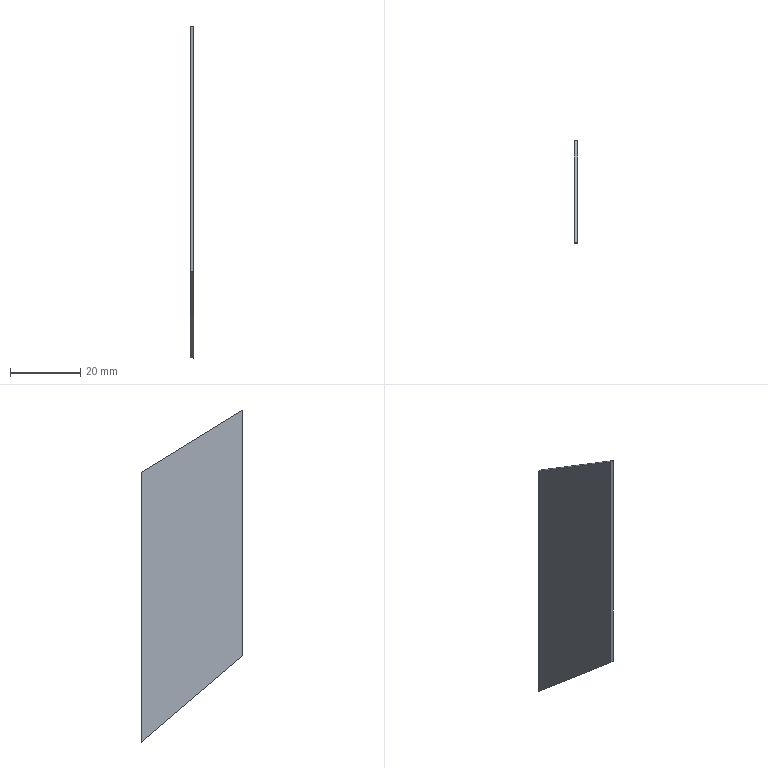Part | STEP file | 09-20 Outlet upper seal plate | 1 solid | 6 faces | box 1 x 29 x 94.448 mm | volume 2126 mm3 | plane 6
STEP:
#1=CARTESIAN_POINT('',(0.,0.,0.));
#2=DIRECTION('',(0.,0.,1.));
#3=DIRECTION('',(1.,0.,0.));
#4=AXIS2_PLACEMENT_3D('',#1,#2,#3);
#5=CARTESIAN_POINT('',(0.,0.,-69.892));
#6=VERTEX_POINT('',#5);
#7=CARTESIAN_POINT('',(1.,0.,-69.892));
#8=VERTEX_POINT('',#7);
#9=CARTESIAN_POINT('',(0.5,0.,-69.892));
#10=DIRECTION('',(1.,0.,0.));
#11=VECTOR('',#10,1.);
#12=LINE('',#9,#11);
#13=CARTESIAN_POINT('',(0.,0.,-69.892));
#14=DIRECTION('',(0.,1.,0.));
#15=DIRECTION('',(0.,0.,1.));
#16=AXIS2_PLACEMENT_3D('',#13,#14,#15);
#17=PLANE('',#16);
#18=CARTESIAN_POINT('',(0.,0.5));
#19=DIRECTION('',(0.,1.));
#20=VECTOR('',#19,1.);
#21=LINE('',#18,#20);
#22=(GEOMETRIC_REPRESENTATION_CONTEXT(2)PARAMETRIC_REPRESENTATION_CONTEXT()REPRESENTATION_CONTEXT('',''));
#23=DEFINITIONAL_REPRESENTATION('',(#21),#22);
#24=PCURVE('',#17,#23);
#25=CARTESIAN_POINT('',(0.,29.,-94.448));
#26=DIRECTION('',(0.,0.6462,0.7632));
#27=DIRECTION('',(0.,-0.7632,0.6462));
#28=AXIS2_PLACEMENT_3D('',#25,#26,#27);
#29=PLANE('',#28);
#30=CARTESIAN_POINT('',(38.,0.5));
#31=DIRECTION('',(0.,1.));
#32=VECTOR('',#31,1.);
#33=LINE('',#30,#32);
#34=(GEOMETRIC_REPRESENTATION_CONTEXT(2)PARAMETRIC_REPRESENTATION_CONTEXT()REPRESENTATION_CONTEXT('',''));
#35=DEFINITIONAL_REPRESENTATION('',(#33),#34);
#36=PCURVE('',#29,#35);
#37=SURFACE_CURVE('',#12,(#24,#36),.PCURVE_S1.);
#38=EDGE_CURVE('',#6,#8,#37,.T.);
#39=ORIENTED_EDGE('',*,*,#38,.T.);
#40=CARTESIAN_POINT('',(1.,0.,0.));
#41=VERTEX_POINT('',#40);
#42=CARTESIAN_POINT('',(1.,0.,-34.946));
#43=DIRECTION('',(0.,0.,-1.));
#44=VECTOR('',#43,1.);
#45=LINE('',#42,#44);
#46=CARTESIAN_POINT('',(34.946,1.));
#47=DIRECTION('',(-1.,0.));
#48=VECTOR('',#47,1.);
#49=LINE('',#46,#48);
#50=(GEOMETRIC_REPRESENTATION_CONTEXT(2)PARAMETRIC_REPRESENTATION_CONTEXT()REPRESENTATION_CONTEXT('',''));
#51=DEFINITIONAL_REPRESENTATION('',(#49),#50);
#52=PCURVE('',#17,#51);
#53=CARTESIAN_POINT('',(1.,0.,-95.015));
#54=DIRECTION('',(-1.,0.,0.));
#55=DIRECTION('',(0.,0.,1.));
#56=AXIS2_PLACEMENT_3D('',#53,#54,#55);
#57=PLANE('',#56);
#58=CARTESIAN_POINT('',(60.069,0.));
#59=DIRECTION('',(-1.,0.));
#60=VECTOR('',#59,1.);
#61=LINE('',#58,#60);
#62=(GEOMETRIC_REPRESENTATION_CONTEXT(2)PARAMETRIC_REPRESENTATION_CONTEXT()REPRESENTATION_CONTEXT('',''));
#63=DEFINITIONAL_REPRESENTATION('',(#61),#62);
#64=PCURVE('',#57,#63);
#65=SURFACE_CURVE('',#45,(#52,#64),.PCURVE_S1.);
#66=EDGE_CURVE('',#41,#8,#65,.T.);
#67=ORIENTED_EDGE('',*,*,#66,.F.);
#68=CARTESIAN_POINT('',(0.,0.,-0.000000012));
#69=VERTEX_POINT('',#68);
#70=CARTESIAN_POINT('',(0.5,0.,0.));
#71=DIRECTION('',(-1.,0.,0.));
#72=VECTOR('',#71,1.);
#73=LINE('',#70,#72);
#74=CARTESIAN_POINT('',(69.892,0.5));
#75=DIRECTION('',(0.,-1.));
#76=VECTOR('',#75,1.);
#77=LINE('',#74,#76);
#78=(GEOMETRIC_REPRESENTATION_CONTEXT(2)PARAMETRIC_REPRESENTATION_CONTEXT()REPRESENTATION_CONTEXT('',''));
#79=DEFINITIONAL_REPRESENTATION('',(#77),#78);
#80=PCURVE('',#17,#79);
#81=CARTESIAN_POINT('',(0.,0.,0.));
#82=DIRECTION('',(0.,-0.522,-0.8529));
#83=DIRECTION('',(0.,0.8529,-0.522));
#84=AXIS2_PLACEMENT_3D('',#81,#82,#83);
#85=PLANE('',#84);
#86=CARTESIAN_POINT('',(0.,0.5));
#87=DIRECTION('',(0.,-1.));
#88=VECTOR('',#87,1.);
#89=LINE('',#86,#88);
#90=(GEOMETRIC_REPRESENTATION_CONTEXT(2)PARAMETRIC_REPRESENTATION_CONTEXT()REPRESENTATION_CONTEXT('',''));
#91=DEFINITIONAL_REPRESENTATION('',(#89),#90);
#92=PCURVE('',#85,#91);
#93=SURFACE_CURVE('',#73,(#80,#92),.PCURVE_S1.);
#94=EDGE_CURVE('',#41,#69,#93,.T.);
#95=ORIENTED_EDGE('',*,*,#94,.T.);
#96=CARTESIAN_POINT('',(0.,0.,-34.946));
#97=DIRECTION('',(0.,0.,1.));
#98=VECTOR('',#97,1.);
#99=LINE('',#96,#98);
#100=CARTESIAN_POINT('',(34.946,0.));
#101=DIRECTION('',(1.,0.));
#102=VECTOR('',#101,1.);
#103=LINE('',#100,#102);
#104=(GEOMETRIC_REPRESENTATION_CONTEXT(2)PARAMETRIC_REPRESENTATION_CONTEXT()REPRESENTATION_CONTEXT('',''));
#105=DEFINITIONAL_REPRESENTATION('',(#103),#104);
#106=PCURVE('',#17,#105);
#107=CARTESIAN_POINT('',(0.,0.,-95.015));
#108=DIRECTION('',(-1.,0.,0.));
#109=DIRECTION('',(0.,0.,1.));
#110=AXIS2_PLACEMENT_3D('',#107,#108,#109);
#111=PLANE('',#110);
#112=CARTESIAN_POINT('',(60.069,0.));
#113=DIRECTION('',(1.,0.));
#114=VECTOR('',#113,1.);
#115=LINE('',#112,#114);
#116=(GEOMETRIC_REPRESENTATION_CONTEXT(2)PARAMETRIC_REPRESENTATION_CONTEXT()REPRESENTATION_CONTEXT('',''));
#117=DEFINITIONAL_REPRESENTATION('',(#115),#116);
#118=PCURVE('',#111,#117);
#119=SURFACE_CURVE('',#99,(#106,#118),.PCURVE_S1.);
#120=EDGE_CURVE('',#6,#69,#119,.T.);
#121=ORIENTED_EDGE('',*,*,#120,.F.);
#122=EDGE_LOOP('',(#39,#67,#95,#121));
#123=FACE_BOUND('',#122,.T.);
#124=ADVANCED_FACE('',(#123),#17,.F.);
#125=CARTESIAN_POINT('',(0.,29.,-17.748));
#126=VERTEX_POINT('',#125);
#127=CARTESIAN_POINT('',(0.,29.,-94.448));
#128=VERTEX_POINT('',#127);
#129=CARTESIAN_POINT('',(0.,29.,-47.224));
#130=DIRECTION('',(0.,0.,-1.));
#131=VECTOR('',#130,1.);
#132=LINE('',#129,#131);
#133=CARTESIAN_POINT('',(47.791,29.));
#134=DIRECTION('',(-1.,0.));
#135=VECTOR('',#134,1.);
#136=LINE('',#133,#135);
#137=(GEOMETRIC_REPRESENTATION_CONTEXT(2)PARAMETRIC_REPRESENTATION_CONTEXT()REPRESENTATION_CONTEXT('',''));
#138=DEFINITIONAL_REPRESENTATION('',(#136),#137);
#139=PCURVE('',#111,#138);
#140=CARTESIAN_POINT('',(0.,29.,-17.748));
#141=DIRECTION('',(0.,-1.,0.));
#142=DIRECTION('',(0.,0.,-1.));
#143=AXIS2_PLACEMENT_3D('',#140,#141,#142);
#144=PLANE('',#143);
#145=CARTESIAN_POINT('',(29.476,0.));
#146=DIRECTION('',(1.,0.));
#147=VECTOR('',#146,1.);
#148=LINE('',#145,#147);
#149=(GEOMETRIC_REPRESENTATION_CONTEXT(2)PARAMETRIC_REPRESENTATION_CONTEXT()REPRESENTATION_CONTEXT('',''));
#150=DEFINITIONAL_REPRESENTATION('',(#148),#149);
#151=PCURVE('',#144,#150);
#152=SURFACE_CURVE('',#132,(#139,#151),.PCURVE_S1.);
#153=EDGE_CURVE('',#126,#128,#152,.T.);
#154=ORIENTED_EDGE('',*,*,#153,.T.);
#155=CARTESIAN_POINT('',(0.,29.,-94.448));
#156=DIRECTION('',(0.,-0.7632,0.6462));
#157=VECTOR('',#156,1.);
#158=LINE('',#155,#157);
#159=CARTESIAN_POINT('',(0.5667,29.));
#160=DIRECTION('',(0.6462,-0.7632));
#161=VECTOR('',#160,1.);
#162=LINE('',#159,#161);
#163=(GEOMETRIC_REPRESENTATION_CONTEXT(2)PARAMETRIC_REPRESENTATION_CONTEXT()REPRESENTATION_CONTEXT('',''));
#164=DEFINITIONAL_REPRESENTATION('',(#162),#163);
#165=PCURVE('',#111,#164);
#166=CARTESIAN_POINT('',(0.000000015,0.));
#167=DIRECTION('',(1.,0.));
#168=VECTOR('',#167,1.);
#169=LINE('',#166,#168);
#170=(GEOMETRIC_REPRESENTATION_CONTEXT(2)PARAMETRIC_REPRESENTATION_CONTEXT()REPRESENTATION_CONTEXT('',''));
#171=DEFINITIONAL_REPRESENTATION('',(#169),#170);
#172=PCURVE('',#29,#171);
#173=SURFACE_CURVE('',#158,(#165,#172),.PCURVE_S1.);
#174=EDGE_CURVE('',#128,#6,#173,.T.);
#175=ORIENTED_EDGE('',*,*,#174,.T.);
#176=ORIENTED_EDGE('',*,*,#120,.T.);
#177=CARTESIAN_POINT('',(0.,0.,-0.000000024));
#178=DIRECTION('',(0.,0.8529,-0.522));
#179=VECTOR('',#178,1.);
#180=LINE('',#177,#179);
#181=CARTESIAN_POINT('',(95.015,0.));
#182=DIRECTION('',(-0.522,0.8529));
#183=VECTOR('',#182,1.);
#184=LINE('',#181,#183);
#185=(GEOMETRIC_REPRESENTATION_CONTEXT(2)PARAMETRIC_REPRESENTATION_CONTEXT()REPRESENTATION_CONTEXT('',''));
#186=DEFINITIONAL_REPRESENTATION('',(#184),#185);
#187=PCURVE('',#111,#186);
#188=CARTESIAN_POINT('',(0.000000012,0.));
#189=DIRECTION('',(1.,0.));
#190=VECTOR('',#189,1.);
#191=LINE('',#188,#190);
#192=(GEOMETRIC_REPRESENTATION_CONTEXT(2)PARAMETRIC_REPRESENTATION_CONTEXT()REPRESENTATION_CONTEXT('',''));
#193=DEFINITIONAL_REPRESENTATION('',(#191),#192);
#194=PCURVE('',#85,#193);
#195=SURFACE_CURVE('',#180,(#187,#194),.PCURVE_S1.);
#196=EDGE_CURVE('',#69,#126,#195,.T.);
#197=ORIENTED_EDGE('',*,*,#196,.T.);
#198=EDGE_LOOP('',(#154,#175,#176,#197));
#199=FACE_BOUND('',#198,.T.);
#200=ADVANCED_FACE('',(#199),#111,.T.);
#201=CARTESIAN_POINT('',(1.,29.,-94.448));
#202=VERTEX_POINT('',#201);
#203=CARTESIAN_POINT('',(1.,29.,-94.448));
#204=DIRECTION('',(0.,-0.7632,0.6462));
#205=VECTOR('',#204,1.);
#206=LINE('',#203,#205);
#207=CARTESIAN_POINT('',(0.5667,29.));
#208=DIRECTION('',(0.6462,-0.7632));
#209=VECTOR('',#208,1.);
#210=LINE('',#207,#209);
#211=(GEOMETRIC_REPRESENTATION_CONTEXT(2)PARAMETRIC_REPRESENTATION_CONTEXT()REPRESENTATION_CONTEXT('',''));
#212=DEFINITIONAL_REPRESENTATION('',(#210),#211);
#213=PCURVE('',#57,#212);
#214=CARTESIAN_POINT('',(0.,1.));
#215=DIRECTION('',(1.,0.));
#216=VECTOR('',#215,1.);
#217=LINE('',#214,#216);
#218=(GEOMETRIC_REPRESENTATION_CONTEXT(2)PARAMETRIC_REPRESENTATION_CONTEXT()REPRESENTATION_CONTEXT('',''));
#219=DEFINITIONAL_REPRESENTATION('',(#217),#218);
#220=PCURVE('',#29,#219);
#221=SURFACE_CURVE('',#206,(#213,#220),.PCURVE_S1.);
#222=EDGE_CURVE('',#202,#8,#221,.T.);
#223=ORIENTED_EDGE('',*,*,#222,.F.);
#224=CARTESIAN_POINT('',(1.,29.,-17.748));
#225=VERTEX_POINT('',#224);
#226=CARTESIAN_POINT('',(1.,29.,-47.224));
#227=DIRECTION('',(0.,0.,-1.));
#228=VECTOR('',#227,1.);
#229=LINE('',#226,#228);
#230=CARTESIAN_POINT('',(47.791,29.));
#231=DIRECTION('',(-1.,0.));
#232=VECTOR('',#231,1.);
#233=LINE('',#230,#232);
#234=(GEOMETRIC_REPRESENTATION_CONTEXT(2)PARAMETRIC_REPRESENTATION_CONTEXT()REPRESENTATION_CONTEXT('',''));
#235=DEFINITIONAL_REPRESENTATION('',(#233),#234);
#236=PCURVE('',#57,#235);
#237=CARTESIAN_POINT('',(29.476,1.));
#238=DIRECTION('',(1.,0.));
#239=VECTOR('',#238,1.);
#240=LINE('',#237,#239);
#241=(GEOMETRIC_REPRESENTATION_CONTEXT(2)PARAMETRIC_REPRESENTATION_CONTEXT()REPRESENTATION_CONTEXT('',''));
#242=DEFINITIONAL_REPRESENTATION('',(#240),#241);
#243=PCURVE('',#144,#242);
#244=SURFACE_CURVE('',#229,(#236,#243),.PCURVE_S1.);
#245=EDGE_CURVE('',#225,#202,#244,.T.);
#246=ORIENTED_EDGE('',*,*,#245,.F.);
#247=CARTESIAN_POINT('',(1.,0.,0.));
#248=DIRECTION('',(0.,0.8529,-0.522));
#249=VECTOR('',#248,1.);
#250=LINE('',#247,#249);
#251=CARTESIAN_POINT('',(95.015,0.));
#252=DIRECTION('',(-0.522,0.8529));
#253=VECTOR('',#252,1.);
#254=LINE('',#251,#253);
#255=(GEOMETRIC_REPRESENTATION_CONTEXT(2)PARAMETRIC_REPRESENTATION_CONTEXT()REPRESENTATION_CONTEXT('',''));
#256=DEFINITIONAL_REPRESENTATION('',(#254),#255);
#257=PCURVE('',#57,#256);
#258=CARTESIAN_POINT('',(0.,1.));
#259=DIRECTION('',(1.,0.));
#260=VECTOR('',#259,1.);
#261=LINE('',#258,#260);
#262=(GEOMETRIC_REPRESENTATION_CONTEXT(2)PARAMETRIC_REPRESENTATION_CONTEXT()REPRESENTATION_CONTEXT('',''));
#263=DEFINITIONAL_REPRESENTATION('',(#261),#262);
#264=PCURVE('',#85,#263);
#265=SURFACE_CURVE('',#250,(#257,#264),.PCURVE_S1.);
#266=EDGE_CURVE('',#41,#225,#265,.T.);
#267=ORIENTED_EDGE('',*,*,#266,.F.);
#268=ORIENTED_EDGE('',*,*,#66,.T.);
#269=EDGE_LOOP('',(#223,#246,#267,#268));
#270=FACE_BOUND('',#269,.T.);
#271=ADVANCED_FACE('',(#270),#57,.F.);
#272=CARTESIAN_POINT('',(0.5,29.,-94.448));
#273=DIRECTION('',(-1.,0.,0.));
#274=VECTOR('',#273,1.);
#275=LINE('',#272,#274);
#276=CARTESIAN_POINT('',(0.,0.5));
#277=DIRECTION('',(0.,-1.));
#278=VECTOR('',#277,1.);
#279=LINE('',#276,#278);
#280=(GEOMETRIC_REPRESENTATION_CONTEXT(2)PARAMETRIC_REPRESENTATION_CONTEXT()REPRESENTATION_CONTEXT('',''));
#281=DEFINITIONAL_REPRESENTATION('',(#279),#280);
#282=PCURVE('',#29,#281);
#283=CARTESIAN_POINT('',(76.7,0.5));
#284=DIRECTION('',(0.,-1.));
#285=VECTOR('',#284,1.);
#286=LINE('',#283,#285);
#287=(GEOMETRIC_REPRESENTATION_CONTEXT(2)PARAMETRIC_REPRESENTATION_CONTEXT()REPRESENTATION_CONTEXT('',''));
#288=DEFINITIONAL_REPRESENTATION('',(#286),#287);
#289=PCURVE('',#144,#288);
#290=SURFACE_CURVE('',#275,(#282,#289),.PCURVE_S1.);
#291=EDGE_CURVE('',#202,#128,#290,.T.);
#292=ORIENTED_EDGE('',*,*,#291,.F.);
#293=ORIENTED_EDGE('',*,*,#222,.T.);
#294=ORIENTED_EDGE('',*,*,#38,.F.);
#295=ORIENTED_EDGE('',*,*,#174,.F.);
#296=EDGE_LOOP('',(#292,#293,#294,#295));
#297=FACE_BOUND('',#296,.T.);
#298=ADVANCED_FACE('',(#297),#29,.F.);
#299=CARTESIAN_POINT('',(0.5,29.,-17.748));
#300=DIRECTION('',(-1.,0.,0.));
#301=VECTOR('',#300,1.);
#302=LINE('',#299,#301);
#303=CARTESIAN_POINT('',(0.,0.5));
#304=DIRECTION('',(0.,-1.));
#305=VECTOR('',#304,1.);
#306=LINE('',#303,#305);
#307=(GEOMETRIC_REPRESENTATION_CONTEXT(2)PARAMETRIC_REPRESENTATION_CONTEXT()REPRESENTATION_CONTEXT('',''));
#308=DEFINITIONAL_REPRESENTATION('',(#306),#307);
#309=PCURVE('',#144,#308);
#310=CARTESIAN_POINT('',(34.,0.5));
#311=DIRECTION('',(0.,-1.));
#312=VECTOR('',#311,1.);
#313=LINE('',#310,#312);
#314=(GEOMETRIC_REPRESENTATION_CONTEXT(2)PARAMETRIC_REPRESENTATION_CONTEXT()REPRESENTATION_CONTEXT('',''));
#315=DEFINITIONAL_REPRESENTATION('',(#313),#314);
#316=PCURVE('',#85,#315);
#317=SURFACE_CURVE('',#302,(#309,#316),.PCURVE_S1.);
#318=EDGE_CURVE('',#225,#126,#317,.T.);
#319=ORIENTED_EDGE('',*,*,#318,.F.);
#320=ORIENTED_EDGE('',*,*,#245,.T.);
#321=ORIENTED_EDGE('',*,*,#291,.T.);
#322=ORIENTED_EDGE('',*,*,#153,.F.);
#323=EDGE_LOOP('',(#319,#320,#321,#322));
#324=FACE_BOUND('',#323,.T.);
#325=ADVANCED_FACE('',(#324),#144,.F.);
#326=ORIENTED_EDGE('',*,*,#94,.F.);
#327=ORIENTED_EDGE('',*,*,#266,.T.);
#328=ORIENTED_EDGE('',*,*,#318,.T.);
#329=ORIENTED_EDGE('',*,*,#196,.F.);
#330=EDGE_LOOP('',(#326,#327,#328,#329));
#331=FACE_BOUND('',#330,.T.);
#332=ADVANCED_FACE('',(#331),#85,.F.);
#333=CLOSED_SHELL('',(#124,#200,#271,#298,#325,#332));
#334=MANIFOLD_SOLID_BREP('',#333);
#335=(LENGTH_UNIT()NAMED_UNIT(*)SI_UNIT(.MILLI.,.METRE.));
#336=UNCERTAINTY_MEASURE_WITH_UNIT(LENGTH_MEASURE(0.0000001),#335,'','');
#337=(NAMED_UNIT(*)PLANE_ANGLE_UNIT()SI_UNIT($,.RADIAN.));
#338=(NAMED_UNIT(*)SI_UNIT($,.STERADIAN.)SOLID_ANGLE_UNIT());
#339=(GEOMETRIC_REPRESENTATION_CONTEXT(3)GLOBAL_UNCERTAINTY_ASSIGNED_CONTEXT((#336))GLOBAL_UNIT_ASSIGNED_CONTEXT((#335,#337,#338))REPRESENTATION_CONTEXT('',''));
#340=ADVANCED_BREP_SHAPE_REPRESENTATION('',(#4,#334),#339);